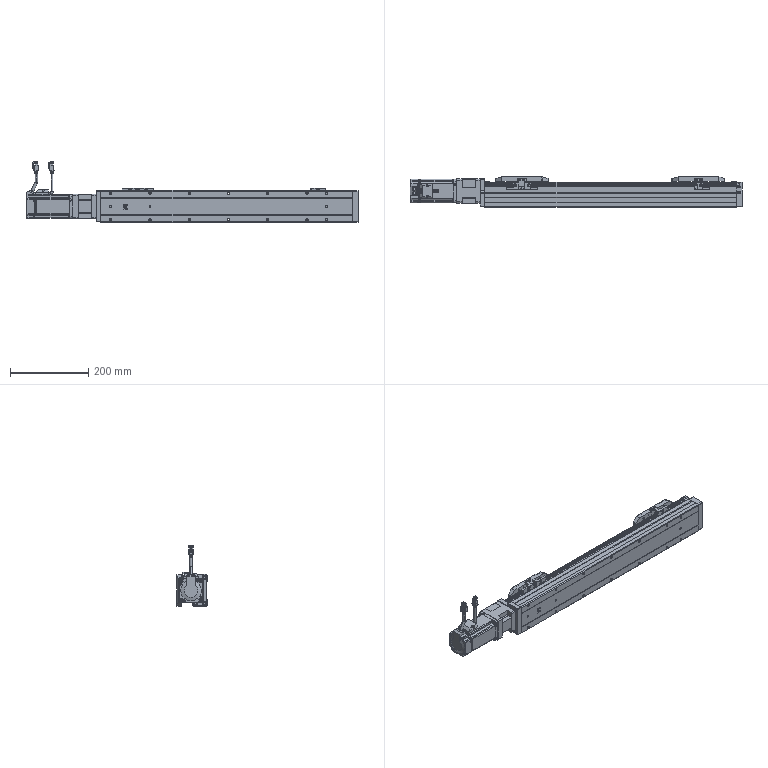Part | SolidWorks | features BaseBody 19 | 19 solids | 2140 faces | box 846 x 78 x 155.983 mm | volume 3838059 mm3 | plane 1343 | cylinder 602 | cone 109 | spline 70 | torus 16 | commonest cylinder face diameters 4 x103 8 x36 1 x34 5.5 x32 5 x28 5.134 x28